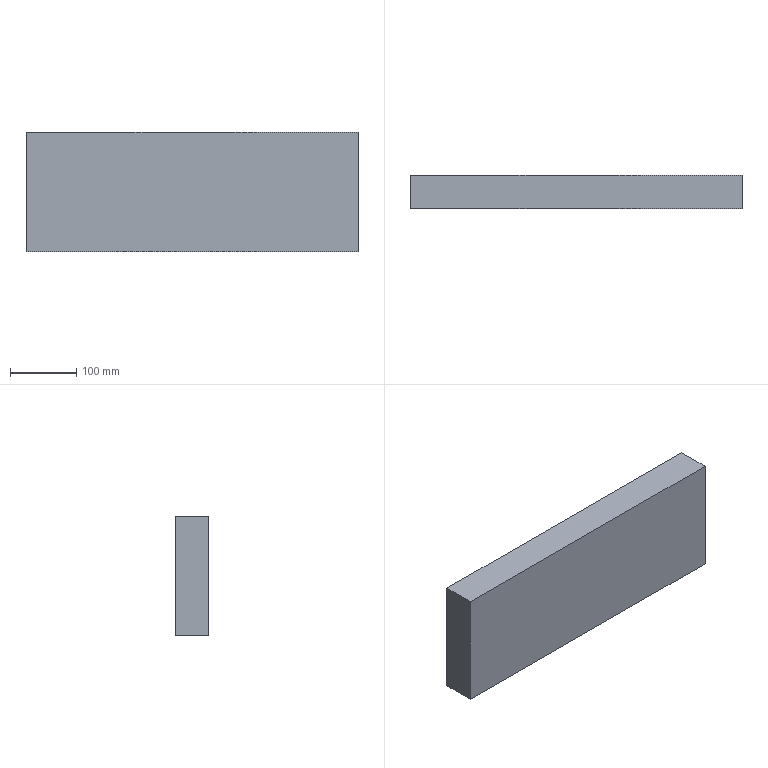Part | SolidWorks | features Extrusion 1 | 1 solid | 6 faces | box 500 x 50 x 180 mm | volume 4500000 mm3 | plane 6
STEP:
#1=CARTESIAN_POINT('',(250.,0.,90.));
#2=VERTEX_POINT('',#1);
#3=CARTESIAN_POINT('',(250.,0.,-90.));
#4=VERTEX_POINT('',#3);
#5=CARTESIAN_POINT('',(250.,0.,-90.));
#6=DIRECTION('',(0.,0.,-1.));
#7=VECTOR('',#6,1000.);
#8=LINE('',#5,#7);
#9=EDGE_CURVE('',#2,#4,#8,.T.);
#10=ORIENTED_EDGE('',*,*,#9,.T.);
#11=CARTESIAN_POINT('',(250.,50.,-90.));
#12=VERTEX_POINT('',#11);
#13=CARTESIAN_POINT('',(250.,50.,-90.));
#14=DIRECTION('',(0.,-1.,0.));
#15=VECTOR('',#14,1000.);
#16=LINE('',#13,#15);
#17=EDGE_CURVE('',#12,#4,#16,.T.);
#18=ORIENTED_EDGE('',*,*,#17,.F.);
#19=CARTESIAN_POINT('',(250.,50.,90.));
#20=VERTEX_POINT('',#19);
#21=CARTESIAN_POINT('',(250.,50.,-90.));
#22=DIRECTION('',(0.,0.,-1.));
#23=VECTOR('',#22,1000.);
#24=LINE('',#21,#23);
#25=EDGE_CURVE('',#20,#12,#24,.T.);
#26=ORIENTED_EDGE('',*,*,#25,.F.);
#27=CARTESIAN_POINT('',(250.,50.,90.));
#28=DIRECTION('',(0.,-1.,0.));
#29=VECTOR('',#28,1000.);
#30=LINE('',#27,#29);
#31=EDGE_CURVE('',#20,#2,#30,.T.);
#32=ORIENTED_EDGE('',*,*,#31,.T.);
#33=EDGE_LOOP('',(#10,#18,#26,#32));
#34=FACE_OUTER_BOUND('',#33,.T.);
#35=CARTESIAN_POINT('',(250.,50.,-90.));
#36=DIRECTION('',(-1.,0.,0.));
#37=DIRECTION('',(0.,0.,1.));
#38=AXIS2_PLACEMENT_3D('',#35,#36,#37);
#39=PLANE('',#38);
#40=ADVANCED_FACE('',(#34),#39,.F.);
#41=CARTESIAN_POINT('',(-250.,0.,-90.));
#42=VERTEX_POINT('',#41);
#43=CARTESIAN_POINT('',(-250.,0.,-90.));
#44=DIRECTION('',(-1.,0.,0.));
#45=VECTOR('',#44,1000.);
#46=LINE('',#43,#45);
#47=EDGE_CURVE('',#4,#42,#46,.T.);
#48=ORIENTED_EDGE('',*,*,#47,.T.);
#49=CARTESIAN_POINT('',(-250.,50.,-90.));
#50=VERTEX_POINT('',#49);
#51=CARTESIAN_POINT('',(-250.,50.,-90.));
#52=DIRECTION('',(0.,-1.,0.));
#53=VECTOR('',#52,1000.);
#54=LINE('',#51,#53);
#55=EDGE_CURVE('',#50,#42,#54,.T.);
#56=ORIENTED_EDGE('',*,*,#55,.F.);
#57=CARTESIAN_POINT('',(-250.,50.,-90.));
#58=DIRECTION('',(-1.,0.,0.));
#59=VECTOR('',#58,1000.);
#60=LINE('',#57,#59);
#61=EDGE_CURVE('',#12,#50,#60,.T.);
#62=ORIENTED_EDGE('',*,*,#61,.F.);
#63=ORIENTED_EDGE('',*,*,#17,.T.);
#64=EDGE_LOOP('',(#48,#56,#62,#63));
#65=FACE_OUTER_BOUND('',#64,.T.);
#66=CARTESIAN_POINT('',(-250.,50.,-90.));
#67=DIRECTION('',(0.,0.,1.));
#68=DIRECTION('',(1.,0.,0.));
#69=AXIS2_PLACEMENT_3D('',#66,#67,#68);
#70=PLANE('',#69);
#71=ADVANCED_FACE('',(#65),#70,.F.);
#72=CARTESIAN_POINT('',(-250.,0.,90.));
#73=VERTEX_POINT('',#72);
#74=CARTESIAN_POINT('',(-250.,0.,-90.));
#75=DIRECTION('',(0.,0.,1.));
#76=VECTOR('',#75,1000.);
#77=LINE('',#74,#76);
#78=EDGE_CURVE('',#42,#73,#77,.T.);
#79=ORIENTED_EDGE('',*,*,#78,.T.);
#80=CARTESIAN_POINT('',(-250.,50.,90.));
#81=VERTEX_POINT('',#80);
#82=CARTESIAN_POINT('',(-250.,50.,90.));
#83=DIRECTION('',(0.,-1.,0.));
#84=VECTOR('',#83,1000.);
#85=LINE('',#82,#84);
#86=EDGE_CURVE('',#81,#73,#85,.T.);
#87=ORIENTED_EDGE('',*,*,#86,.F.);
#88=CARTESIAN_POINT('',(-250.,50.,-90.));
#89=DIRECTION('',(0.,0.,1.));
#90=VECTOR('',#89,1000.);
#91=LINE('',#88,#90);
#92=EDGE_CURVE('',#50,#81,#91,.T.);
#93=ORIENTED_EDGE('',*,*,#92,.F.);
#94=ORIENTED_EDGE('',*,*,#55,.T.);
#95=EDGE_LOOP('',(#79,#87,#93,#94));
#96=FACE_OUTER_BOUND('',#95,.T.);
#97=CARTESIAN_POINT('',(-250.,50.,-90.));
#98=DIRECTION('',(1.,0.,0.));
#99=DIRECTION('',(0.,0.,-1.));
#100=AXIS2_PLACEMENT_3D('',#97,#98,#99);
#101=PLANE('',#100);
#102=ADVANCED_FACE('',(#96),#101,.F.);
#103=CARTESIAN_POINT('',(-250.,0.,90.));
#104=DIRECTION('',(1.,0.,0.));
#105=VECTOR('',#104,1000.);
#106=LINE('',#103,#105);
#107=EDGE_CURVE('',#73,#2,#106,.T.);
#108=ORIENTED_EDGE('',*,*,#107,.T.);
#109=ORIENTED_EDGE('',*,*,#31,.F.);
#110=CARTESIAN_POINT('',(-250.,50.,90.));
#111=DIRECTION('',(1.,0.,0.));
#112=VECTOR('',#111,1000.);
#113=LINE('',#110,#112);
#114=EDGE_CURVE('',#81,#20,#113,.T.);
#115=ORIENTED_EDGE('',*,*,#114,.F.);
#116=ORIENTED_EDGE('',*,*,#86,.T.);
#117=EDGE_LOOP('',(#108,#109,#115,#116));
#118=FACE_OUTER_BOUND('',#117,.T.);
#119=CARTESIAN_POINT('',(-250.,50.,90.));
#120=DIRECTION('',(0.,0.,-1.));
#121=DIRECTION('',(-1.,0.,0.));
#122=AXIS2_PLACEMENT_3D('',#119,#120,#121);
#123=PLANE('',#122);
#124=ADVANCED_FACE('',(#118),#123,.F.);
#125=ORIENTED_EDGE('',*,*,#25,.T.);
#126=ORIENTED_EDGE('',*,*,#61,.T.);
#127=ORIENTED_EDGE('',*,*,#92,.T.);
#128=ORIENTED_EDGE('',*,*,#114,.T.);
#129=EDGE_LOOP('',(#125,#126,#127,#128));
#130=FACE_OUTER_BOUND('',#129,.T.);
#131=CARTESIAN_POINT('',(0.,50.,0.));
#132=DIRECTION('',(0.,1.,0.));
#133=DIRECTION('',(0.,0.,1.));
#134=AXIS2_PLACEMENT_3D('',#131,#132,#133);
#135=PLANE('',#134);
#136=ADVANCED_FACE('',(#130),#135,.T.);
#137=ORIENTED_EDGE('',*,*,#9,.F.);
#138=ORIENTED_EDGE('',*,*,#107,.F.);
#139=ORIENTED_EDGE('',*,*,#78,.F.);
#140=ORIENTED_EDGE('',*,*,#47,.F.);
#141=EDGE_LOOP('',(#137,#138,#139,#140));
#142=FACE_OUTER_BOUND('',#141,.T.);
#143=CARTESIAN_POINT('',(0.,0.,0.));
#144=DIRECTION('',(0.,1.,0.));
#145=DIRECTION('',(0.,0.,1.));
#146=AXIS2_PLACEMENT_3D('',#143,#144,#145);
#147=PLANE('',#146);
#148=ADVANCED_FACE('',(#142),#147,.F.);
#149=CLOSED_SHELL('',(#40,#71,#102,#124,#136,#148));
#150=MANIFOLD_SOLID_BREP('',#149);
#151=CARTESIAN_POINT('',(0.,0.,0.));
#152=DIRECTION('',(0.,0.,1.));
#153=DIRECTION('',(1.,0.,0.));
#154=AXIS2_PLACEMENT_3D('',#151,#152,#153);
#155=(LENGTH_UNIT()NAMED_UNIT(*)SI_UNIT(.MILLI.,.METRE.));
#156=UNCERTAINTY_MEASURE_WITH_UNIT(LENGTH_MEASURE(0.00001),#155,'','');
#157=(NAMED_UNIT(*)PLANE_ANGLE_UNIT()SI_UNIT($,.RADIAN.));
#158=(NAMED_UNIT(*)SI_UNIT($,.STERADIAN.)SOLID_ANGLE_UNIT());
#159=(GEOMETRIC_REPRESENTATION_CONTEXT(3)GLOBAL_UNCERTAINTY_ASSIGNED_CONTEXT((#156))GLOBAL_UNIT_ASSIGNED_CONTEXT((#155,#157,#158))REPRESENTATION_CONTEXT('',''));
#160=ADVANCED_BREP_SHAPE_REPRESENTATION('',(#150,#154),#159);